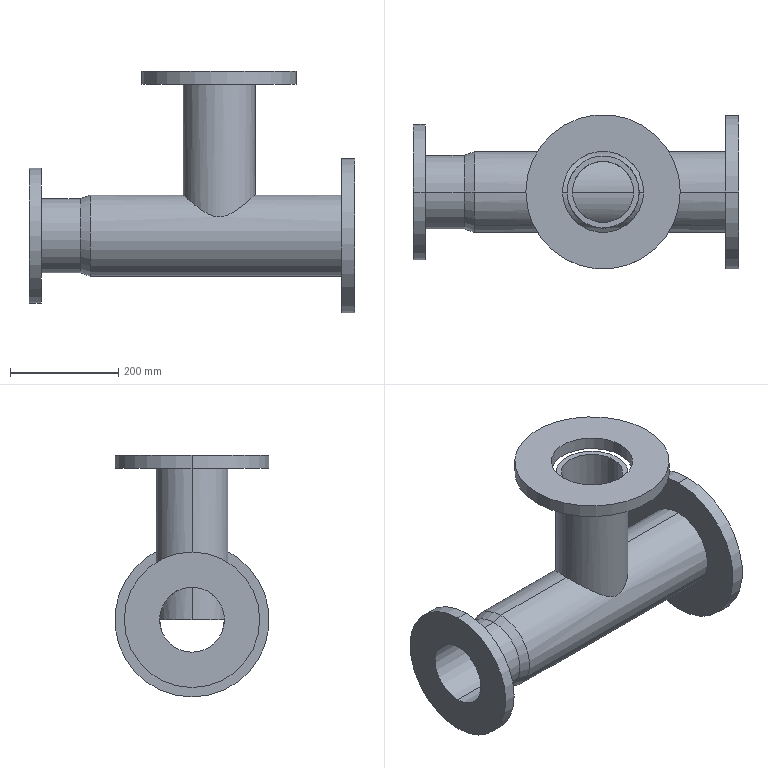Part | SolidWorks | features ICE 2, Revolution 1 | 2 solids | 37 faces | box 600 x 285 x 446.5 mm | volume 7468872 mm3 | cylinder 27 | plane 8 | cone 2 | commonest cylinder face diameters 150 x6 133 x5 113 x4 120 x4 285 x4 136.6 x2